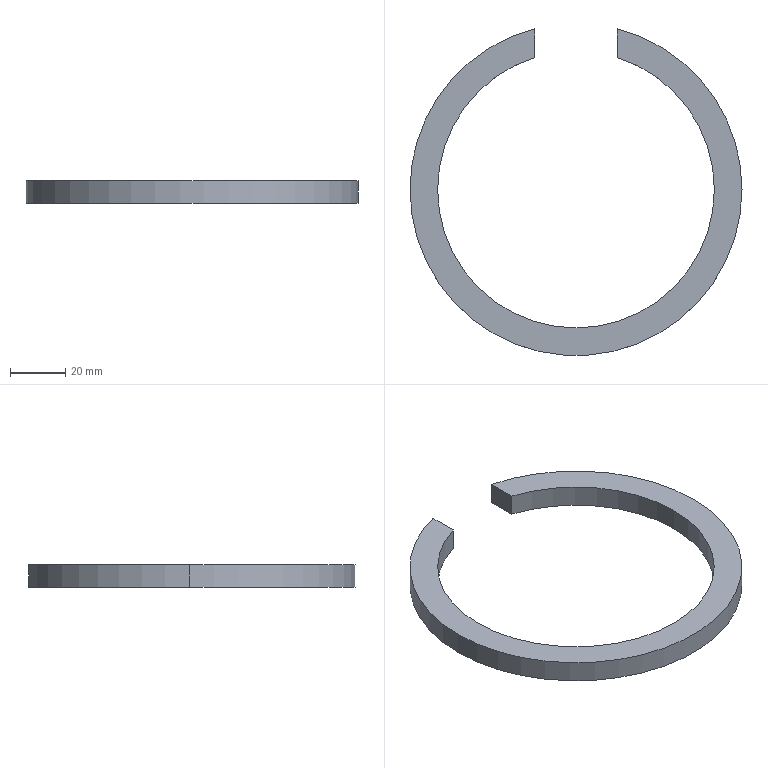Part | SolidWorks | features Extrusion 1, ICE 1 | 1 solid | 10 faces | box 120 x 118.095 x 8 mm | volume 25215 mm3 | cylinder 6 | plane 4 | commonest cylinder face diameters 100 x3 120 x3
STEP:
#1=CARTESIAN_POINT('',(-50.,0.,8.));
#2=VERTEX_POINT('',#1);
#3=CARTESIAN_POINT('',(50.,0.,8.));
#4=VERTEX_POINT('',#3);
#5=CARTESIAN_POINT('',(0.,0.,8.));
#6=DIRECTION('',(0.,0.,1.));
#7=DIRECTION('',(1.,0.,0.));
#8=AXIS2_PLACEMENT_3D('',#5,#6,#7);
#9=CIRCLE('',#8,50.);
#10=EDGE_CURVE('',#2,#4,#9,.T.);
#11=ORIENTED_EDGE('',*,*,#10,.T.);
#12=CARTESIAN_POINT('',(50.,0.,0.));
#13=VERTEX_POINT('',#12);
#14=CARTESIAN_POINT('',(50.,0.,8.));
#15=DIRECTION('',(0.,0.,-1.));
#16=VECTOR('',#15,1000.);
#17=LINE('',#14,#16);
#18=EDGE_CURVE('',#4,#13,#17,.T.);
#19=ORIENTED_EDGE('',*,*,#18,.T.);
#20=CARTESIAN_POINT('',(-50.,0.,0.));
#21=VERTEX_POINT('',#20);
#22=CARTESIAN_POINT('',(0.,0.,0.));
#23=DIRECTION('',(0.,0.,1.));
#24=DIRECTION('',(1.,0.,0.));
#25=AXIS2_PLACEMENT_3D('',#22,#23,#24);
#26=CIRCLE('',#25,50.);
#27=EDGE_CURVE('',#21,#13,#26,.T.);
#28=ORIENTED_EDGE('',*,*,#27,.F.);
#29=CARTESIAN_POINT('',(-50.,0.,8.));
#30=DIRECTION('',(0.,0.,-1.));
#31=VECTOR('',#30,1000.);
#32=LINE('',#29,#31);
#33=EDGE_CURVE('',#2,#21,#32,.T.);
#34=ORIENTED_EDGE('',*,*,#33,.F.);
#35=EDGE_LOOP('',(#11,#19,#28,#34));
#36=FACE_OUTER_BOUND('',#35,.T.);
#37=CARTESIAN_POINT('',(0.,0.,8.));
#38=DIRECTION('',(0.,0.,-1.));
#39=DIRECTION('',(-1.,0.,0.));
#40=AXIS2_PLACEMENT_3D('',#37,#38,#39);
#41=CYLINDRICAL_SURFACE('',#40,50.);
#42=ADVANCED_FACE('',(#36),#41,.F.);
#43=CARTESIAN_POINT('',(-15.,47.697,8.));
#44=VERTEX_POINT('',#43);
#45=CARTESIAN_POINT('',(0.,0.,8.));
#46=DIRECTION('',(0.,0.,1.));
#47=DIRECTION('',(1.,0.,0.));
#48=AXIS2_PLACEMENT_3D('',#45,#46,#47);
#49=CIRCLE('',#48,50.);
#50=EDGE_CURVE('',#44,#2,#49,.T.);
#51=ORIENTED_EDGE('',*,*,#50,.T.);
#52=ORIENTED_EDGE('',*,*,#33,.T.);
#53=CARTESIAN_POINT('',(-15.,47.697,0.));
#54=VERTEX_POINT('',#53);
#55=CARTESIAN_POINT('',(0.,0.,0.));
#56=DIRECTION('',(0.,0.,1.));
#57=DIRECTION('',(1.,0.,0.));
#58=AXIS2_PLACEMENT_3D('',#55,#56,#57);
#59=CIRCLE('',#58,50.);
#60=EDGE_CURVE('',#54,#21,#59,.T.);
#61=ORIENTED_EDGE('',*,*,#60,.F.);
#62=CARTESIAN_POINT('',(-15.,47.697,8.));
#63=DIRECTION('',(0.,0.,-1.));
#64=VECTOR('',#63,1000.);
#65=LINE('',#62,#64);
#66=EDGE_CURVE('',#44,#54,#65,.T.);
#67=ORIENTED_EDGE('',*,*,#66,.F.);
#68=EDGE_LOOP('',(#51,#52,#61,#67));
#69=FACE_OUTER_BOUND('',#68,.T.);
#70=CARTESIAN_POINT('',(0.,0.,8.));
#71=DIRECTION('',(0.,0.,-1.));
#72=DIRECTION('',(-1.,0.,0.));
#73=AXIS2_PLACEMENT_3D('',#70,#71,#72);
#74=CYLINDRICAL_SURFACE('',#73,50.);
#75=ADVANCED_FACE('',(#69),#74,.F.);
#76=CARTESIAN_POINT('',(60.,0.,8.));
#77=VERTEX_POINT('',#76);
#78=CARTESIAN_POINT('',(15.,58.095,8.));
#79=VERTEX_POINT('',#78);
#80=CARTESIAN_POINT('',(0.,0.,8.));
#81=DIRECTION('',(0.,0.,1.));
#82=DIRECTION('',(1.,0.,0.));
#83=AXIS2_PLACEMENT_3D('',#80,#81,#82);
#84=CIRCLE('',#83,60.);
#85=EDGE_CURVE('',#77,#79,#84,.T.);
#86=ORIENTED_EDGE('',*,*,#85,.F.);
#87=CARTESIAN_POINT('',(60.,0.,0.));
#88=VERTEX_POINT('',#87);
#89=CARTESIAN_POINT('',(60.,0.,8.));
#90=DIRECTION('',(0.,0.,-1.));
#91=VECTOR('',#90,1000.);
#92=LINE('',#89,#91);
#93=EDGE_CURVE('',#77,#88,#92,.T.);
#94=ORIENTED_EDGE('',*,*,#93,.T.);
#95=CARTESIAN_POINT('',(15.,58.095,0.));
#96=VERTEX_POINT('',#95);
#97=CARTESIAN_POINT('',(0.,0.,0.));
#98=DIRECTION('',(0.,0.,1.));
#99=DIRECTION('',(1.,0.,0.));
#100=AXIS2_PLACEMENT_3D('',#97,#98,#99);
#101=CIRCLE('',#100,60.);
#102=EDGE_CURVE('',#88,#96,#101,.T.);
#103=ORIENTED_EDGE('',*,*,#102,.T.);
#104=CARTESIAN_POINT('',(15.,58.095,8.));
#105=DIRECTION('',(0.,0.,1.));
#106=VECTOR('',#105,1000.);
#107=LINE('',#104,#106);
#108=EDGE_CURVE('',#96,#79,#107,.T.);
#109=ORIENTED_EDGE('',*,*,#108,.T.);
#110=EDGE_LOOP('',(#86,#94,#103,#109));
#111=FACE_OUTER_BOUND('',#110,.T.);
#112=CARTESIAN_POINT('',(0.,0.,8.));
#113=DIRECTION('',(0.,0.,-1.));
#114=DIRECTION('',(-1.,0.,0.));
#115=AXIS2_PLACEMENT_3D('',#112,#113,#114);
#116=CYLINDRICAL_SURFACE('',#115,60.);
#117=ADVANCED_FACE('',(#111),#116,.T.);
#118=ORIENTED_EDGE('',*,*,#93,.F.);
#119=CARTESIAN_POINT('',(-60.,0.,8.));
#120=VERTEX_POINT('',#119);
#121=CARTESIAN_POINT('',(0.,0.,8.));
#122=DIRECTION('',(0.,0.,1.));
#123=DIRECTION('',(1.,0.,0.));
#124=AXIS2_PLACEMENT_3D('',#121,#122,#123);
#125=CIRCLE('',#124,60.);
#126=EDGE_CURVE('',#120,#77,#125,.T.);
#127=ORIENTED_EDGE('',*,*,#126,.F.);
#128=CARTESIAN_POINT('',(-60.,0.,0.));
#129=VERTEX_POINT('',#128);
#130=CARTESIAN_POINT('',(-60.,0.,8.));
#131=DIRECTION('',(0.,0.,-1.));
#132=VECTOR('',#131,1000.);
#133=LINE('',#130,#132);
#134=EDGE_CURVE('',#120,#129,#133,.T.);
#135=ORIENTED_EDGE('',*,*,#134,.T.);
#136=CARTESIAN_POINT('',(0.,0.,0.));
#137=DIRECTION('',(0.,0.,1.));
#138=DIRECTION('',(1.,0.,0.));
#139=AXIS2_PLACEMENT_3D('',#136,#137,#138);
#140=CIRCLE('',#139,60.);
#141=EDGE_CURVE('',#129,#88,#140,.T.);
#142=ORIENTED_EDGE('',*,*,#141,.T.);
#143=EDGE_LOOP('',(#118,#127,#135,#142));
#144=FACE_OUTER_BOUND('',#143,.T.);
#145=CARTESIAN_POINT('',(0.,0.,8.));
#146=DIRECTION('',(0.,0.,-1.));
#147=DIRECTION('',(-1.,0.,0.));
#148=AXIS2_PLACEMENT_3D('',#145,#146,#147);
#149=CYLINDRICAL_SURFACE('',#148,60.);
#150=ADVANCED_FACE('',(#144),#149,.T.);
#151=CARTESIAN_POINT('',(15.,47.697,8.));
#152=VERTEX_POINT('',#151);
#153=CARTESIAN_POINT('',(15.,15.58,8.));
#154=DIRECTION('',(0.,1.,0.));
#155=VECTOR('',#154,1000.);
#156=LINE('',#153,#155);
#157=EDGE_CURVE('',#152,#79,#156,.T.);
#158=ORIENTED_EDGE('',*,*,#157,.F.);
#159=CARTESIAN_POINT('',(0.,0.,8.));
#160=DIRECTION('',(0.,0.,1.));
#161=DIRECTION('',(1.,0.,0.));
#162=AXIS2_PLACEMENT_3D('',#159,#160,#161);
#163=CIRCLE('',#162,50.);
#164=EDGE_CURVE('',#4,#152,#163,.T.);
#165=ORIENTED_EDGE('',*,*,#164,.F.);
#166=ORIENTED_EDGE('',*,*,#10,.F.);
#167=ORIENTED_EDGE('',*,*,#50,.F.);
#168=CARTESIAN_POINT('',(-15.,58.095,8.));
#169=VERTEX_POINT('',#168);
#170=CARTESIAN_POINT('',(-15.,15.58,8.));
#171=DIRECTION('',(0.,-1.,0.));
#172=VECTOR('',#171,1000.);
#173=LINE('',#170,#172);
#174=EDGE_CURVE('',#169,#44,#173,.T.);
#175=ORIENTED_EDGE('',*,*,#174,.F.);
#176=CARTESIAN_POINT('',(0.,0.,8.));
#177=DIRECTION('',(0.,0.,1.));
#178=DIRECTION('',(1.,0.,0.));
#179=AXIS2_PLACEMENT_3D('',#176,#177,#178);
#180=CIRCLE('',#179,60.);
#181=EDGE_CURVE('',#169,#120,#180,.T.);
#182=ORIENTED_EDGE('',*,*,#181,.T.);
#183=ORIENTED_EDGE('',*,*,#126,.T.);
#184=ORIENTED_EDGE('',*,*,#85,.T.);
#185=EDGE_LOOP('',(#158,#165,#166,#167,#175,#182,#183,#184));
#186=FACE_OUTER_BOUND('',#185,.T.);
#187=CARTESIAN_POINT('',(0.,0.,8.));
#188=DIRECTION('',(0.,0.,1.));
#189=DIRECTION('',(1.,0.,0.));
#190=AXIS2_PLACEMENT_3D('',#187,#188,#189);
#191=PLANE('',#190);
#192=ADVANCED_FACE('',(#186),#191,.T.);
#193=ORIENTED_EDGE('',*,*,#60,.T.);
#194=ORIENTED_EDGE('',*,*,#27,.T.);
#195=CARTESIAN_POINT('',(15.,47.697,0.));
#196=VERTEX_POINT('',#195);
#197=CARTESIAN_POINT('',(0.,0.,0.));
#198=DIRECTION('',(0.,0.,1.));
#199=DIRECTION('',(1.,0.,0.));
#200=AXIS2_PLACEMENT_3D('',#197,#198,#199);
#201=CIRCLE('',#200,50.);
#202=EDGE_CURVE('',#13,#196,#201,.T.);
#203=ORIENTED_EDGE('',*,*,#202,.T.);
#204=CARTESIAN_POINT('',(15.,0.,0.));
#205=DIRECTION('',(0.,1.,0.));
#206=VECTOR('',#205,1000.);
#207=LINE('',#204,#206);
#208=EDGE_CURVE('',#196,#96,#207,.T.);
#209=ORIENTED_EDGE('',*,*,#208,.T.);
#210=ORIENTED_EDGE('',*,*,#102,.F.);
#211=ORIENTED_EDGE('',*,*,#141,.F.);
#212=CARTESIAN_POINT('',(-15.,58.095,0.));
#213=VERTEX_POINT('',#212);
#214=CARTESIAN_POINT('',(0.,0.,0.));
#215=DIRECTION('',(0.,0.,1.));
#216=DIRECTION('',(1.,0.,0.));
#217=AXIS2_PLACEMENT_3D('',#214,#215,#216);
#218=CIRCLE('',#217,60.);
#219=EDGE_CURVE('',#213,#129,#218,.T.);
#220=ORIENTED_EDGE('',*,*,#219,.F.);
#221=CARTESIAN_POINT('',(-15.,0.,0.));
#222=DIRECTION('',(0.,-1.,0.));
#223=VECTOR('',#222,1000.);
#224=LINE('',#221,#223);
#225=EDGE_CURVE('',#213,#54,#224,.T.);
#226=ORIENTED_EDGE('',*,*,#225,.T.);
#227=EDGE_LOOP('',(#193,#194,#203,#209,#210,#211,#220,#226));
#228=FACE_OUTER_BOUND('',#227,.T.);
#229=CARTESIAN_POINT('',(0.,0.,0.));
#230=DIRECTION('',(0.,0.,1.));
#231=DIRECTION('',(1.,0.,0.));
#232=AXIS2_PLACEMENT_3D('',#229,#230,#231);
#233=PLANE('',#232);
#234=ADVANCED_FACE('',(#228),#233,.F.);
#235=ORIENTED_EDGE('',*,*,#134,.F.);
#236=ORIENTED_EDGE('',*,*,#181,.F.);
#237=CARTESIAN_POINT('',(-15.,58.095,8.));
#238=DIRECTION('',(0.,0.,-1.));
#239=VECTOR('',#238,1000.);
#240=LINE('',#237,#239);
#241=EDGE_CURVE('',#169,#213,#240,.T.);
#242=ORIENTED_EDGE('',*,*,#241,.T.);
#243=ORIENTED_EDGE('',*,*,#219,.T.);
#244=EDGE_LOOP('',(#235,#236,#242,#243));
#245=FACE_OUTER_BOUND('',#244,.T.);
#246=CARTESIAN_POINT('',(0.,0.,8.));
#247=DIRECTION('',(0.,0.,-1.));
#248=DIRECTION('',(-1.,0.,0.));
#249=AXIS2_PLACEMENT_3D('',#246,#247,#248);
#250=CYLINDRICAL_SURFACE('',#249,60.);
#251=ADVANCED_FACE('',(#245),#250,.T.);
#252=ORIENTED_EDGE('',*,*,#18,.F.);
#253=ORIENTED_EDGE('',*,*,#164,.T.);
#254=CARTESIAN_POINT('',(15.,47.697,8.));
#255=DIRECTION('',(0.,0.,1.));
#256=VECTOR('',#255,1000.);
#257=LINE('',#254,#256);
#258=EDGE_CURVE('',#196,#152,#257,.T.);
#259=ORIENTED_EDGE('',*,*,#258,.F.);
#260=ORIENTED_EDGE('',*,*,#202,.F.);
#261=EDGE_LOOP('',(#252,#253,#259,#260));
#262=FACE_OUTER_BOUND('',#261,.T.);
#263=CARTESIAN_POINT('',(0.,0.,8.));
#264=DIRECTION('',(0.,0.,-1.));
#265=DIRECTION('',(-1.,0.,0.));
#266=AXIS2_PLACEMENT_3D('',#263,#264,#265);
#267=CYLINDRICAL_SURFACE('',#266,50.);
#268=ADVANCED_FACE('',(#262),#267,.F.);
#269=ORIENTED_EDGE('',*,*,#174,.T.);
#270=ORIENTED_EDGE('',*,*,#66,.T.);
#271=ORIENTED_EDGE('',*,*,#225,.F.);
#272=ORIENTED_EDGE('',*,*,#241,.F.);
#273=EDGE_LOOP('',(#269,#270,#271,#272));
#274=FACE_OUTER_BOUND('',#273,.T.);
#275=CARTESIAN_POINT('',(-15.,15.58,-7.));
#276=DIRECTION('',(-1.,0.,0.));
#277=DIRECTION('',(0.,0.,1.));
#278=AXIS2_PLACEMENT_3D('',#275,#276,#277);
#279=PLANE('',#278);
#280=ADVANCED_FACE('',(#274),#279,.F.);
#281=ORIENTED_EDGE('',*,*,#208,.F.);
#282=ORIENTED_EDGE('',*,*,#258,.T.);
#283=ORIENTED_EDGE('',*,*,#157,.T.);
#284=ORIENTED_EDGE('',*,*,#108,.F.);
#285=EDGE_LOOP('',(#281,#282,#283,#284));
#286=FACE_OUTER_BOUND('',#285,.T.);
#287=CARTESIAN_POINT('',(15.,15.58,-7.));
#288=DIRECTION('',(1.,0.,0.));
#289=DIRECTION('',(0.,0.,-1.));
#290=AXIS2_PLACEMENT_3D('',#287,#288,#289);
#291=PLANE('',#290);
#292=ADVANCED_FACE('',(#286),#291,.F.);
#293=CLOSED_SHELL('',(#42,#75,#117,#150,#192,#234,#251,#268,#280,#292));
#294=MANIFOLD_SOLID_BREP('',#293);
#295=CARTESIAN_POINT('',(0.,0.,0.));
#296=DIRECTION('',(0.,0.,1.));
#297=DIRECTION('',(1.,0.,0.));
#298=AXIS2_PLACEMENT_3D('',#295,#296,#297);
#299=(LENGTH_UNIT()NAMED_UNIT(*)SI_UNIT(.MILLI.,.METRE.));
#300=UNCERTAINTY_MEASURE_WITH_UNIT(LENGTH_MEASURE(0.00001),#299,'','');
#301=(NAMED_UNIT(*)PLANE_ANGLE_UNIT()SI_UNIT($,.RADIAN.));
#302=(NAMED_UNIT(*)SI_UNIT($,.STERADIAN.)SOLID_ANGLE_UNIT());
#303=(GEOMETRIC_REPRESENTATION_CONTEXT(3)GLOBAL_UNCERTAINTY_ASSIGNED_CONTEXT((#300))GLOBAL_UNIT_ASSIGNED_CONTEXT((#299,#301,#302))REPRESENTATION_CONTEXT('',''));
#304=ADVANCED_BREP_SHAPE_REPRESENTATION('',(#294,#298),#303);